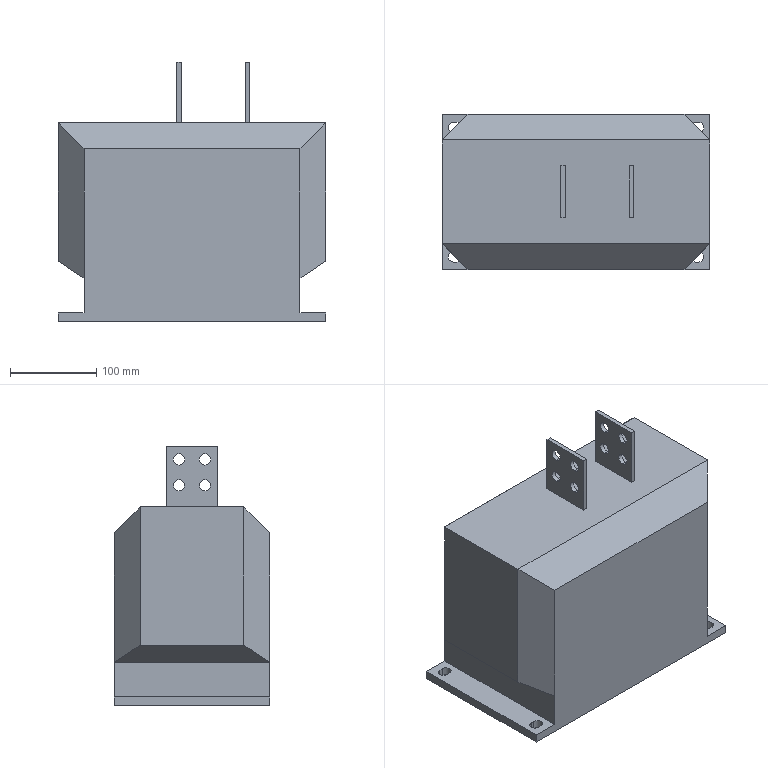Part | STEP file | 921272131 | 1 solid | 66 faces | box 310 x 180 x 300 mm | volume 11781247 mm3 | plane 38 | cylinder 28 | commonest cylinder face diameters 13 x16 12 x12